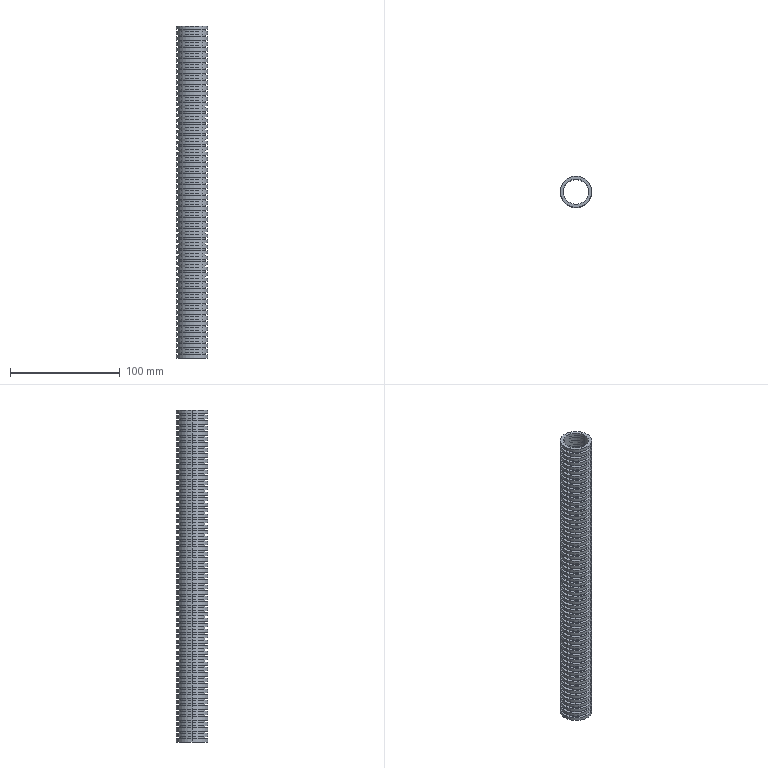Part | STEP file | P0177567_EZT_SCHUTZSCHLAUCH_MKR-23-PG-21.2_1 | 1 solid | 366 faces | box 28.5 x 28.5 x 303 mm | volume 45141 mm3 | cylinder 244 | plane 122 | commonest cylinder face diameters 28.5 x122 24 x120 23 x2